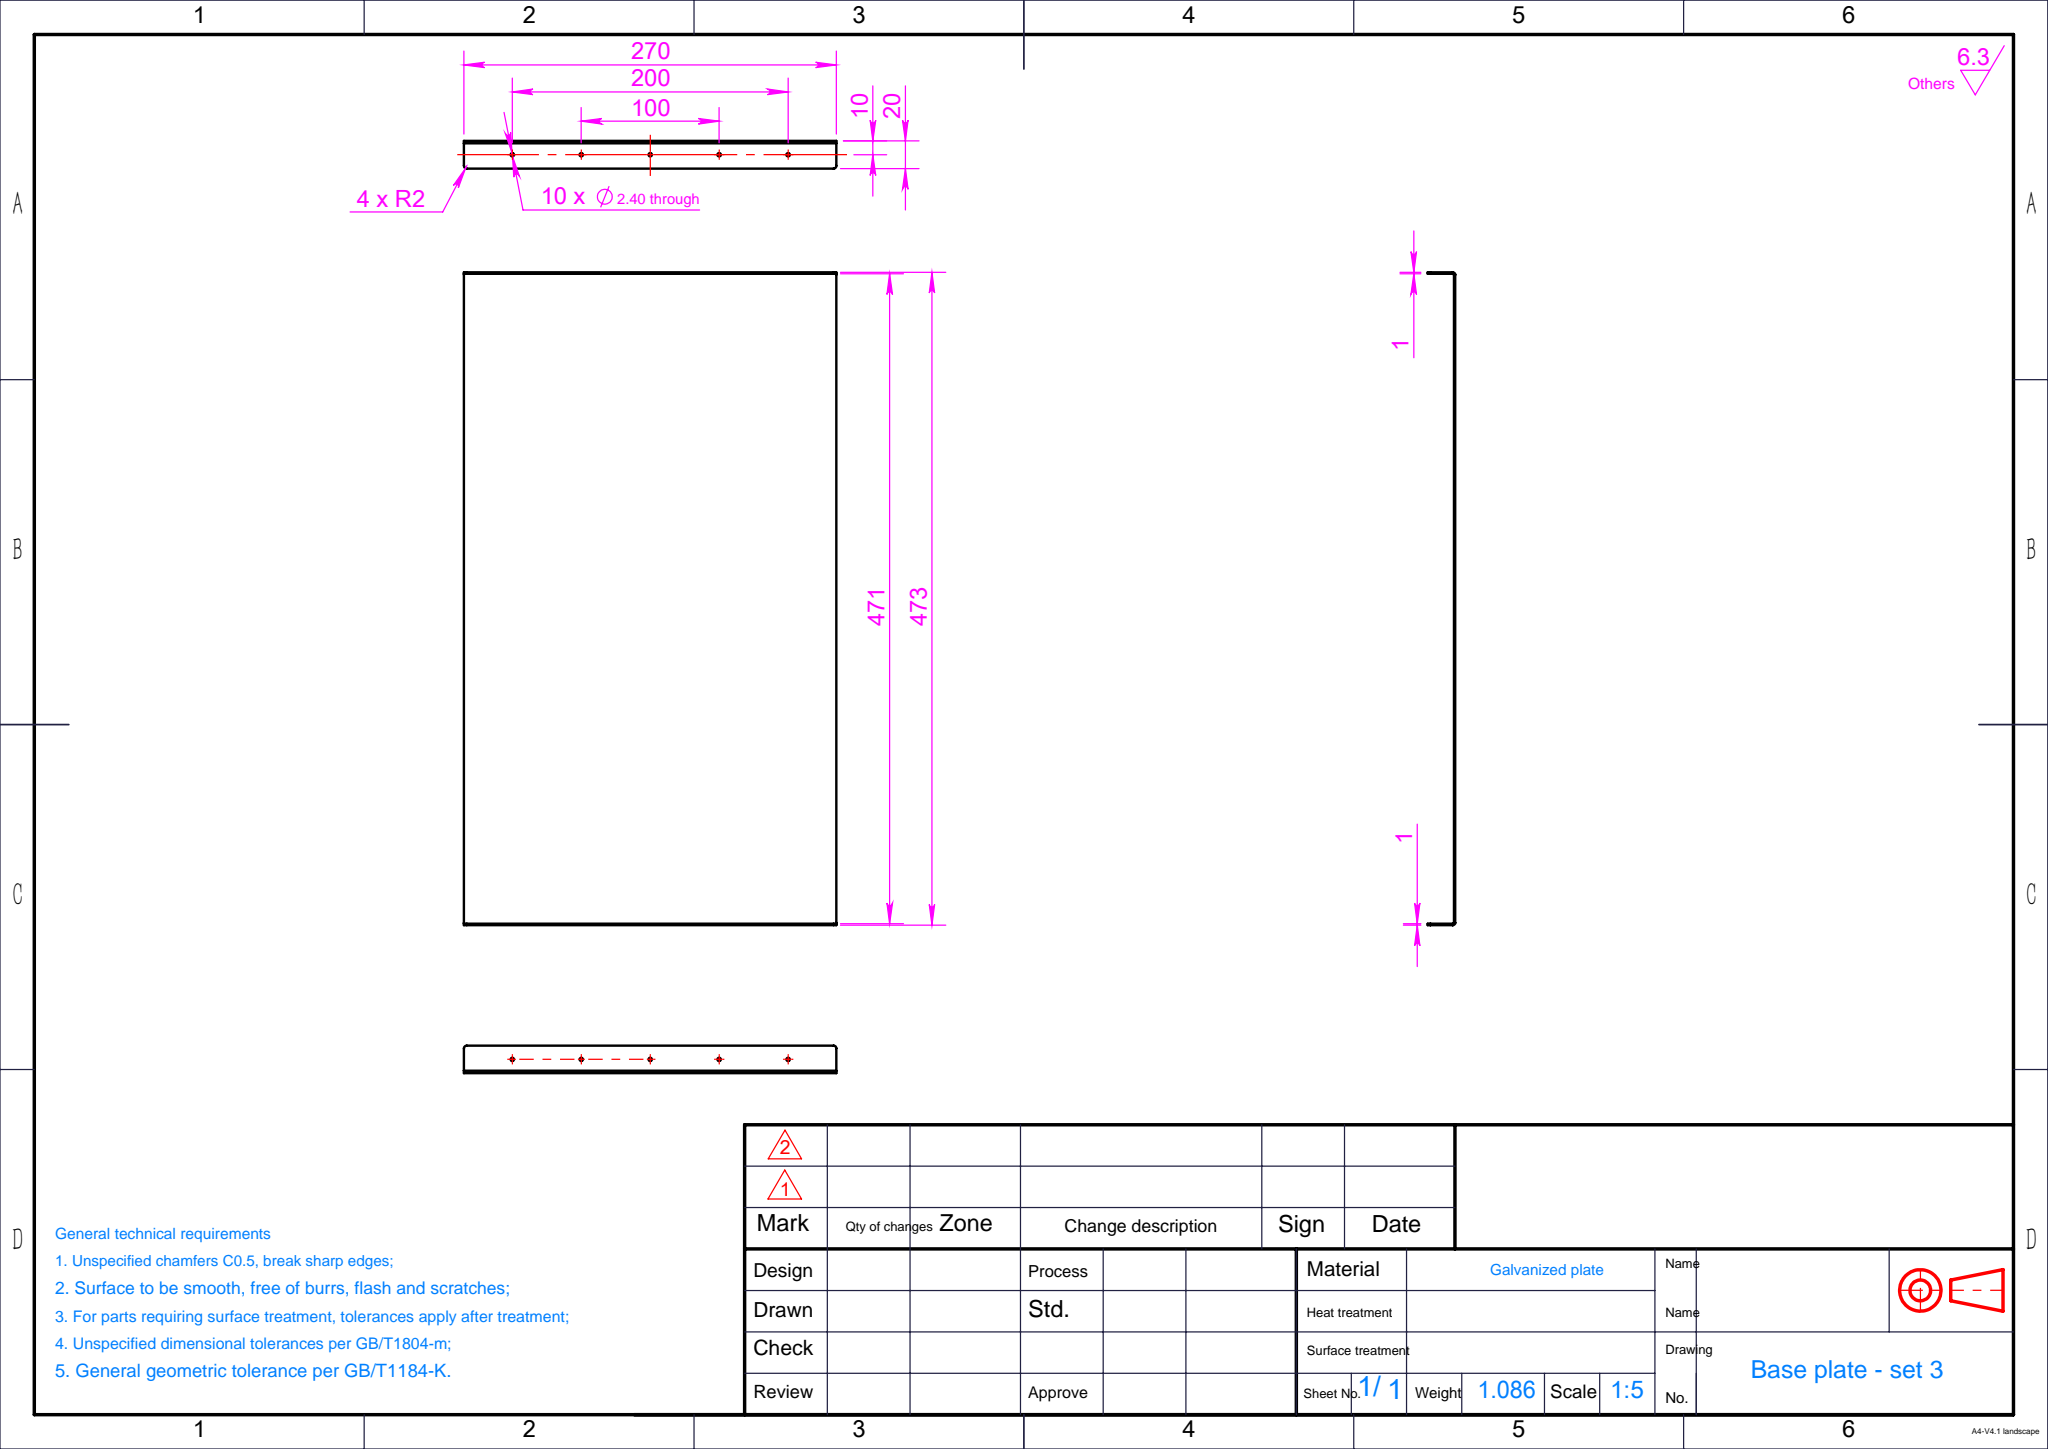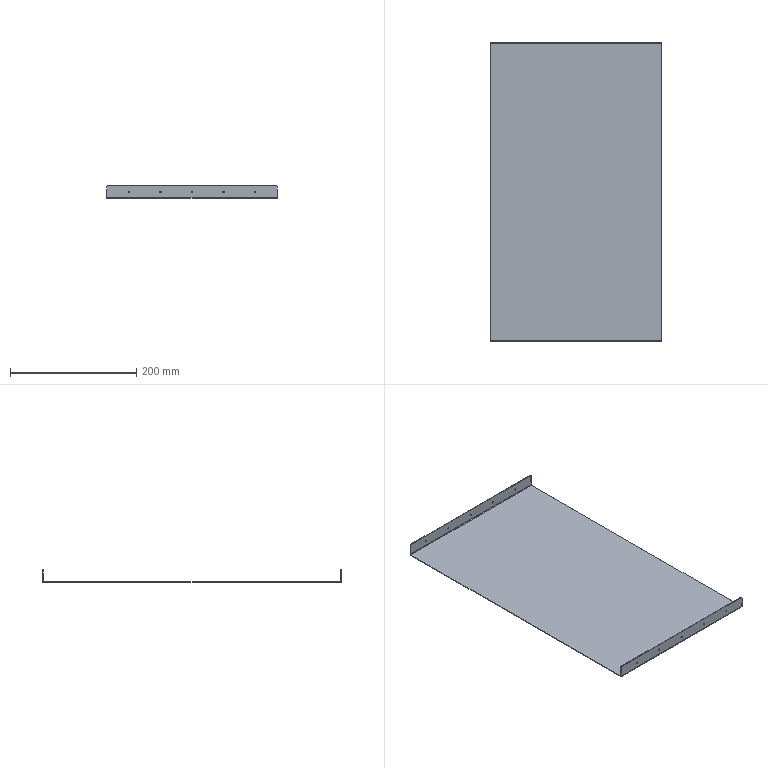Part | SolidWorks | features 3DProfileFeature 1, EdgeFlange 1, Fillet 1, FlatPattern 1, HoleWzd 1, LPattern 1, MirrorPattern 1, SMBaseFlange 1, SheetMetal 1 | 1 solid | 46 faces | box 270 x 473 x 20 mm | volume 137635 mm3 | cylinder 28 | plane 18 | commonest cylinder face diameters 2.4 x20 4 x4 1.473 x2 3.473 x2